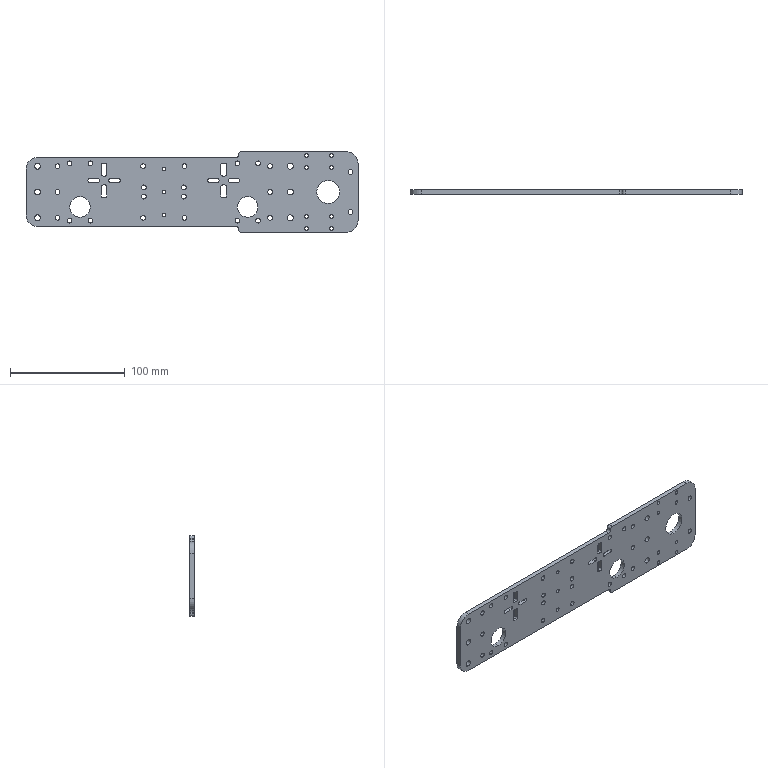Part | SolidWorks | features BaseBody 1 | 1 solid | 154 faces | box 289 x 4 x 70 mm | volume 66384 mm3 | cylinder 120 | plane 34 | commonest cylinder face diameters 3.2 x46 4.2 x32 4 x16 5.2 x12 20 x6 4.4 x4